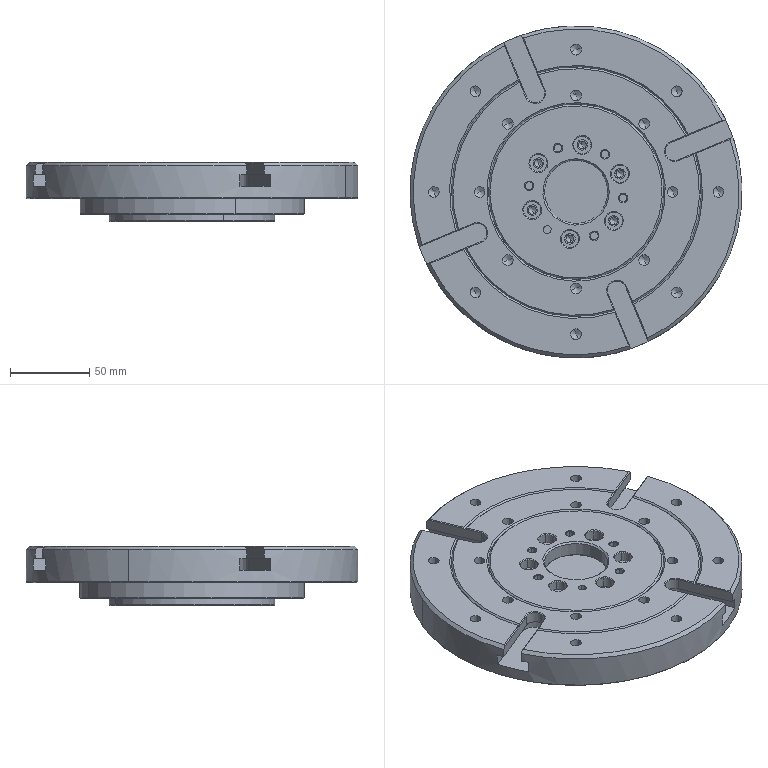NC program | Mastercam | posted with a generic post
Lines 1 to 959 of 19401:
%
:0001()
(MATERIAL - ALUMINUM MM - 2024)
(T1|25 BNOS |H1|D1|WEAR COMP|TOOL DIA. - 25.|XY STOCK TO LEAVE - .15|Z STOCK TO LEAVE - .1)
(T3|10 CHM |H3)
(T4|8.5 DR |H4)
(T5|14 FEM |H5)
(T6|6.8 DR |H6)
(T7|M8 X 1.25 RH |H7)
N100 G21
N102 G0 G17 G40 G80 G90 G94 G98
N104 G0 G28 G91 Z0.
N106 G0 G28 X0. Y0.
(25 BNOS |TOOL - 1|DIA. OFF. - 1|LEN. - 1|TOOL DIA. - 25.)
N108 T1 M6
N110 G0 G54 G90 X1.154 Y47.25 C0. B0. S2300 M3
N112 G43 H1 Z62.5
N114 Z14.2
N116 G1 Z12.708 F2000.
N118 G41 D1 Y28.5 F3500.
N120 Y8.5
N122 G40 Y-10.25
N124 Z12.215 F2000.
N126 G42 D1 Y8.5 F3500.
N128 Y28.5
N130 G40 Y47.25
N132 Z11.723 F2000.
N134 G41 D1 Y28.5 F3500.
N136 Y8.5
N138 G40 Y-10.25
N140 Z11.231 F2000.
N142 G42 D1 Y8.5 F3500.
N144 Y28.5
N146 G40 Y47.25
N148 Z10.738 F2000.
N150 G41 D1 Y28.5 F3500.
N152 Y8.5
N154 G40 Y-10.25
N156 Z10.246 F2000.
N158 G42 D1 Y8.5 F3500.
N160 Y28.5
N162 G40 Y47.25
N164 Z9.754 F2000.
N166 G41 D1 Y28.5 F3500.
N168 Y8.5
N170 G40 Y-10.25
N172 Z9.262 F2000.
N174 G42 D1 Y8.5 F3500.
N176 Y28.5
N178 G40 Y47.25
N180 Z8.769 F2000.
N182 G41 D1 Y28.5 F3500.
N184 Y8.5
N186 G40 Y-10.25
N188 Z8.277 F2000.
N190 G42 D1 Y8.5 F3500.
N192 Y28.5
N194 G40 Y47.25
N196 Z7.785 F2000.
N198 G41 D1 Y28.5 F3500.
N200 Y8.5
N202 G40 Y-10.25
N204 Z7.292 F2000.
N206 G42 D1 Y8.5 F3500.
N208 Y28.5
N210 G40 Y47.25
N212 Z6.8 F2000.
N214 G41 D1 Y28.5 F3500.
N216 Y8.5
N218 G40 Y-10.25
N220 Z6.308 F2000.
N222 G42 D1 Y8.5 F3500.
N224 Y28.5
N226 G40 Y47.25
N228 Z5.815 F2000.
N230 G41 D1 Y28.5 F3500.
N232 Y8.5
N234 G40 Y-10.25
N236 Z5.323 F2000.
N238 G42 D1 Y8.5 F3500.
N240 Y28.5
N242 G40 Y47.25
N244 Z4.831 F2000.
N246 G41 D1 Y28.5 F3500.
N248 Y8.5
N250 G40 Y-10.25
N252 Z4.338 F2000.
N254 G42 D1 Y8.5 F3500.
N256 Y28.5
N258 G40 Y47.25
N260 Z3.846 F2000.
N262 G41 D1 Y28.5 F3500.
N264 Y8.5
N266 G40 Y-10.25
N268 Z3.354 F2000.
N270 G42 D1 Y8.5 F3500.
N272 Y28.5
N274 G40 Y47.25
N276 Z2.862 F2000.
N278 G41 D1 Y28.5 F3500.
N280 Y8.5
N282 G40 Y-10.25
N284 Z2.369 F2000.
N286 G42 D1 Y8.5 F3500.
N288 Y28.5
N290 G40 Y47.25
N292 Z1.877 F2000.
N294 G41 D1 Y28.5 F3500.
N296 Y8.5
N298 G40 Y-10.25
N300 Z1.385 F2000.
N302 G42 D1 Y8.5 F3500.
N304 Y28.5
N306 G40 Y47.25
N308 Z.892 F2000.
N310 G41 D1 Y28.5 F3500.
N312 Y8.5
N314 G40 Y-10.25
N316 Z.4 F2000.
N318 G42 D1 Y8.5 F3500.
N320 Y28.5
N322 G40 Y47.25
N324 Z-.092 F2000.
N326 G41 D1 Y28.5 F3500.
N328 Y8.5
N330 G40 Y-10.25
N332 Z-.585 F2000.
N334 G42 D1 Y8.5 F3500.
N336 Y28.5
N338 G40 Y47.25
N340 Z-1.077 F2000.
N342 G41 D1 Y28.5 F3500.
N344 Y8.5
N346 G40 Y-10.25
N348 Z-1.569 F2000.
N350 G42 D1 Y8.5 F3500.
N352 Y28.5
N354 G40 Y47.25
N356 Z-2.062 F2000.
N358 G41 D1 Y28.5 F3500.
N360 Y8.5
N362 G40 Y-10.25
N364 Z-2.554 F2000.
N366 G42 D1 Y8.5 F3500.
N368 Y28.5
N370 G40 Y47.25
N372 Z-3.046 F2000.
N374 G41 D1 Y28.5 F3500.
N376 Y8.5
N378 G40 Y-10.25
N380 Z-3.538 F2000.
N382 G42 D1 Y8.5 F3500.
N384 Y28.5
N386 G40 Y47.25
N388 Z-4.031 F2000.
N390 G41 D1 Y28.5 F3500.
N392 Y8.5
N394 G40 Y-10.25
N396 Z-4.523 F2000.
N398 G42 D1 Y8.5 F3500.
N400 Y28.5
N402 G40 Y47.25
N404 Z-5.015 F2000.
N406 G41 D1 Y28.5 F3500.
N408 Y8.5
N410 G40 Y-10.25
N412 Z-5.508 F2000.
N414 G42 D1 Y8.5 F3500.
N416 Y28.5
N418 G40 Y47.25
N420 Z-6. F2000.
N422 G41 D1 Y28.5 F3500.
N424 Y8.5
N426 G40 Y-10.25
N428 Z-6.492 F2000.
N430 G42 D1 Y8.5 F3500.
N432 Y28.5
N434 G40 Y47.25
N436 Z-6.985 F2000.
N438 G41 D1 Y28.5 F3500.
N440 Y8.5
N442 G40 Y-10.25
N444 Z-7.477 F2000.
N446 G42 D1 Y8.5 F3500.
N448 Y28.5
N450 G40 Y47.25
N452 Z-7.969 F2000.
N454 G41 D1 Y28.5 F3500.
N456 Y8.5
N458 G40 Y-10.25
N460 Z-8.462 F2000.
N462 G42 D1 Y8.5 F3500.
N464 Y28.5
N466 G40 Y47.25
N468 Z-8.954 F2000.
N470 G41 D1 Y28.5 F3500.
N472 Y8.5
N474 G40 Y-10.25
N476 Z-9.446 F2000.
N478 G42 D1 Y8.5 F3500.
N480 Y28.5
N482 G40 Y47.25
N484 Z-9.938 F2000.
N486 G41 D1 Y28.5 F3500.
N488 Y8.5
N490 G40 Y-10.25
N492 Z-10.431 F2000.
N494 G42 D1 Y8.5 F3500.
N496 Y28.5
N498 G40 Y47.25
N500 Z-10.923 F2000.
N502 G41 D1 Y28.5 F3500.
N504 Y8.5
N506 G40 Y-10.25
N508 Z-11.415 F2000.
N510 G42 D1 Y8.5 F3500.
N512 Y28.5
N514 G40 Y47.25
N516 Z-11.908 F2000.
N518 G41 D1 Y28.5 F3500.
N520 Y8.5
N522 G40 Y-10.25
N524 Z-12.4 F2000.
N526 G42 D1 Y8.5 F3500.
N528 Y28.5
N530 G40 Y47.25
N532 G0 Z62.5
N534 S3500 M3
N536 X21.899 Y-5.5
N538 Z16.907
N540 G1 Z11.907 F2000.
N542 Y8.5
N544 Y28.5
N546 Y42.5
N548 X21.847
N550 Z11.715
N552 Y28.5
N554 Y8.5
N556 Y-5.5
N558 X21.795
N560 Z11.522
N562 Y8.5
N564 Y28.5
N566 Y42.5
N568 X21.744
N570 Z11.33
N572 Y28.5
N574 Y8.5
N576 Y-5.5
N578 X21.692
N580 Z11.138
N582 Y8.5
N584 Y28.5
N586 Y42.5
N588 X21.641
N590 Z10.946
N592 Y28.5
N594 Y8.5
N596 Y-5.5
N598 X21.589
N600 Z10.753
N602 Y8.5
N604 Y28.5
N606 Y42.5
N608 X21.538
N610 Z10.561
N612 Y28.5
N614 Y8.5
N616 Y-5.5
N618 X21.486
N620 Z10.369
N622 Y8.5
N624 Y28.5
N626 Y42.5
N628 X21.435
N630 Z10.176
N632 Y28.5
N634 Y8.5
N636 Y-5.5
N638 X21.383
N640 Z9.984
N642 Y8.5
N644 Y28.5
N646 Y42.5
N648 X21.332
N650 Z9.792
N652 Y28.5
N654 Y8.5
N656 Y-5.5
N658 X21.28
N660 Z9.599
N662 Y8.5
N664 Y28.5
N666 Y42.5
N668 X21.229
N670 Z9.407
N672 Y28.5
N674 Y8.5
N676 Y-5.5
N678 X21.177
N680 Z9.215
N682 Y8.5
N684 Y28.5
N686 Y42.5
N688 X21.126
N690 Z9.022
N692 Y28.5
N694 Y8.5
N696 Y-5.5
N698 X21.074
N700 Z8.83
N702 Y8.5
N704 Y28.5
N706 Y42.5
N708 X21.023
N710 Z8.638
N712 Y28.5
N714 Y8.5
N716 Y-5.5
N718 X20.971
N720 Z8.446
N722 Y8.5
N724 Y28.5
N726 Y42.5
N728 X20.919
N730 Z8.253
N732 Y28.5
N734 Y8.5
N736 Y-5.5
N738 X20.868
N740 Z8.061
N742 Y8.5
N744 Y28.5
N746 Y42.5
N748 X20.816
N750 Z7.869
N752 Y28.5
N754 Y8.5
N756 Y-5.5
N758 X20.765
N760 Z7.676
N762 Y8.5
N764 Y28.5
N766 Y42.5
N768 X20.713
N770 Z7.484
N772 Y28.5
N774 Y8.5
N776 Y-5.5
N778 X20.662
N780 Z7.292
N782 Y8.5
N784 Y28.5
N786 Y42.5
N788 X20.61
N790 Z7.099
N792 Y28.5
N794 Y8.5
N796 Y-5.5
N798 X20.559
N800 Z6.907
N802 Y8.5
N804 Y28.5
N806 Y42.5
N808 X20.507
N810 Z6.715
N812 Y28.5
N814 Y8.5
N816 Y-5.5
N818 X20.456
N820 Z6.522
N822 Y8.5
N824 Y28.5
N826 Y42.5
N828 X20.404
N830 Z6.33
N832 Y28.5
N834 Y8.5
N836 Y-5.5
N838 X20.353
N840 Z6.138
N842 Y8.5
N844 Y28.5
N846 Y42.5
N848 X20.301
N850 Z5.946
N852 Y28.5
N854 Y8.5
N856 Y-5.5
N858 X20.25
N860 Z5.753
N862 Y8.5
N864 Y28.5
N866 Y42.5
N868 X20.198
N870 Z5.561
N872 Y28.5
N874 Y8.5
N876 Y-5.5
N878 X20.147
N880 Z5.369
N882 Y8.5
N884 Y28.5
N886 Y42.5
N888 X20.095
N890 Z5.176
N892 Y28.5
N894 Y8.5
N896 Y-5.5
N898 X20.043
N900 Z4.984
N902 Y8.5
N904 Y28.5
N906 Y42.5
N908 X19.992
N910 Z4.792
N912 Y28.5
N914 Y8.5
N916 Y-5.5
N918 X19.94
N920 Z4.599
N922 Y8.5
N924 Y28.5
N926 Y42.5
N928 X19.889
N930 Z4.407
N932 Y28.5
N934 Y8.5
N936 Y-5.5
N938 X19.837
N940 Z4.215
N942 Y8.5
N944 Y28.5
N946 Y42.5
N948 X19.786
N950 Z4.022
N952 Y28.5
N954 Y8.5
N956 Y-5.5
N958 X19.734
N960 Z3.83
N962 Y8.5
N964 Y28.5
N966 Y42.5
N968 X19.683
N970 Z3.638
N972 Y28.5
N974 Y8.5
N976 Y-5.5
N978 X19.631
N980 Z3.446
N982 Y8.5
N984 Y28.5
N986 Y42.5
N988 X19.58
N990 Z3.253
N992 Y28.5
N994 Y8.5
N996 Y-5.5
N998 X19.528
N1000 Z3.061
N1002 Y8.5
N1004 Y28.5
N1006 Y42.5
N1008 X19.477
N1010 Z2.869
N1012 Y28.5
N1014 Y8.5
N1016 Y-5.5
N1018 X19.425
N1020 Z2.676
N1022 Y8.5
N1024 Y28.5
N1026 Y42.5
N1028 X19.374
N1030 Z2.484
N1032 Y28.5
N1034 Y8.5
N1036 Y-5.5
N1038 X19.322
N1040 Z2.292
N1042 Y8.5
N1044 Y28.5
N1046 Y42.5
N1048 X19.271
N1050 Z2.099
N1052 Y28.5
N1054 Y8.5
N1056 Y-5.5
N1058 X19.219
N1060 Z1.907
N1062 Y8.5
N1064 Y28.5
N1066 Y42.5
N1068 X19.168
N1070 Z1.715
N1072 Y28.5
N1074 Y8.5
N1076 Y-5.5
N1078 X19.116
N1080 Z1.522
N1082 Y8.5
N1084 Y28.5
N1086 Y42.5
N1088 X19.064
N1090 Z1.33
N1092 Y28.5
N1094 Y8.5
N1096 Y-5.5
N1098 X19.013
N1100 Z1.138
N1102 Y8.5
N1104 Y28.5
N1106 Y42.5
N1108 X18.961
N1110 Z.946
N1112 Y28.5
N1114 Y8.5
N1116 Y-5.5
N1118 X18.91
N1120 Z.753
N1122 Y8.5
N1124 Y28.5
N1126 Y42.5
N1128 X18.858
N1130 Z.561
N1132 Y28.5
N1134 Y8.5
N1136 Y-5.5
N1138 X18.807
N1140 Z.369
N1142 Y8.5
N1144 Y28.5
N1146 Y42.5
N1148 X18.755
N1150 Z.176
N1152 Y28.5
N1154 Y8.5
N1156 Y-5.5
N1158 X18.704
N1160 Z-.016
N1162 Y8.5
N1164 Y28.5
N1166 Y42.5
N1168 X18.652
N1170 Z-.208
N1172 Y28.5
N1174 Y8.5
N1176 Y-5.5
N1178 X18.601
N1180 Z-.401
N1182 Y8.5
N1184 Y28.5
N1186 Y42.5
N1188 X18.549
N1190 Z-.593
N1192 Y28.5
N1194 Y8.5
N1196 Y-5.5
N1198 X18.498
N1200 Z-.785
N1202 Y8.5
N1204 Y28.5
N1206 Y42.5
N1208 X18.446
N1210 Z-.978
N1212 Y28.5
N1214 Y8.5
N1216 Y-5.5
N1218 X18.395
N1220 Z-1.17
N1222 Y8.5
N1224 Y28.5
N1226 Y42.5
N1228 X18.343
N1230 Z-1.362
N1232 Y28.5
N1234 Y8.5
N1236 Y-5.5
N1238 X18.292
N1240 Z-1.554
N1242 Y8.5
N1244 Y28.5
N1246 Y42.5
N1248 X18.24
N1250 Z-1.747
N1252 Y28.5
N1254 Y8.5
N1256 Y-5.5
N1258 X18.188
N1260 Z-1.939
N1262 Y8.5
N1264 Y28.5
N1266 Y42.5
N1268 X18.137
N1270 Z-2.131
N1272 Y28.5
N1274 Y8.5
N1276 Y-5.5
N1278 X18.085
N1280 Z-2.324
N1282 Y8.5
N1284 Y28.5
N1286 Y42.5
N1288 X18.034
N1290 Z-2.516
N1292 Y28.5
N1294 Y8.5
N1296 Y-5.5
N1298 X17.982
N1300 Z-2.708
N1302 Y8.5
N1304 Y28.5
N1306 Y42.5
N1308 X17.931
N1310 Z-2.901
N1312 Y28.5
N1314 Y8.5
N1316 Y-5.5
N1318 X17.879
N1320 Z-3.093
N1322 Y8.5
N1324 Y28.5
N1326 Y42.5
N1328 X17.828
N1330 Z-3.285
N1332 Y28.5
N1334 Y8.5
N1336 Y-5.5
N1338 X17.776
N1340 Z-3.478
N1342 Y8.5
N1344 Y28.5
N1346 Y42.5
N1348 X17.725
N1350 Z-3.67
N1352 Y28.5
N1354 Y8.5
N1356 Y-5.5
N1358 X17.673
N1360 Z-3.862
N1362 Y8.5
N1364 Y28.5
N1366 Y42.5
N1368 X17.622
N1370 Z-4.054
N1372 Y28.5
N1374 Y8.5
N1376 Y-5.5
N1378 X17.57
N1380 Z-4.247
N1382 Y8.5
N1384 Y28.5
N1386 Y42.5
N1388 X17.519
N1390 Z-4.439
N1392 Y28.5
N1394 Y8.5
N1396 Y-5.5
N1398 X17.467
N1400 Z-4.631
N1402 Y8.5
N1404 Y28.5
N1406 Y42.5
N1408 X17.416
N1410 Z-4.824
N1412 Y28.5
N1414 Y8.5
N1416 Y-5.5
N1418 X17.364
N1420 Z-5.016
N1422 Y8.5
N1424 Y28.5
N1426 Y42.5
N1428 X17.312
N1430 Z-5.208
N1432 Y28.5
N1434 Y8.5
N1436 Y-5.5
N1438 X17.261
N1440 Z-5.401
N1442 Y8.5
N1444 Y28.5
N1446 Y42.5
N1448 X17.209
N1450 Z-5.593
N1452 Y28.5
N1454 Y8.5
N1456 Y-5.5
N1458 X17.158
N1460 Z-5.785
N1462 Y8.5
N1464 Y28.5
N1466 Y42.5
N1468 X17.106
N1470 Z-5.978
N1472 Y28.5
N1474 Y8.5
N1476 Y-5.5
N1478 X17.055
N1480 Z-6.17
N1482 Y8.5
N1484 Y28.5
N1486 Y42.5
N1488 X17.003
N1490 Z-6.362
N1492 Y28.5
N1494 Y8.5
N1496 Y-5.5
N1498 X16.952
N1500 Z-6.554
N1502 Y8.5
N1504 Y28.5
N1506 Y42.5
N1508 X16.9
N1510 Z-6.747
N1512 Y28.5
N1514 Y8.5
N1516 Y-5.5
N1518 X16.849
N1520 Z-6.939
N1522 Y8.5
N1524 Y28.5
N1526 Y42.5
N1528 X16.797
N1530 Z-7.131
N1532 Y28.5
N1534 Y8.5
N1536 Y-5.5
N1538 X16.746
N1540 Z-7.324
N1542 Y8.5
N1544 Y28.5
N1546 Y42.5
N1548 X16.694
N1550 Z-7.516
N1552 Y28.5
N1554 Y8.5
N1556 Y-5.5
N1558 X16.643
N1560 Z-7.708
N1562 Y8.5
N1564 Y28.5
N1566 Y42.5
N1568 X16.591
N1570 Z-7.901
N1572 Y28.5
N1574 Y8.5
N1576 Y-5.5
N1578 X16.54
N1580 Z-8.093
N1582 Y8.5
N1584 Y28.5
N1586 Y42.5
N1588 X16.488
N1590 Z-8.285
N1592 Y28.5
N1594 Y8.5
N1596 Y-5.5
N1598 X16.436
N1600 Z-8.478
N1602 Y8.5
N1604 Y28.5
N1606 Y42.5
N1608 X16.385
N1610 Z-8.67
N1612 Y28.5
N1614 Y8.5
N1616 Y-5.5
N1618 X16.333
N1620 Z-8.862
N1622 Y8.5
N1624 Y28.5
N1626 Y42.5
N1628 X16.282
N1630 Z-9.054
N1632 Y28.5
N1634 Y8.5
N1636 Y-5.5
N1638 X16.23
N1640 Z-9.247
N1642 Y8.5
N1644 Y28.5
N1646 Y42.5
N1648 X16.179
N1650 Z-9.439
N1652 Y28.5
N1654 Y8.5
N1656 Y-5.5
N1658 X16.127
N1660 Z-9.631
N1662 Y8.5
N1664 Y28.5
N1666 Y42.5
N1668 X16.076
N1670 Z-9.824
N1672 Y28.5
N1674 Y8.5
N1676 Y-5.5
N1678 X16.024
N1680 Z-10.016
N1682 Y8.5
N1684 Y28.5
N1686 Y42.5
N1688 X15.973
N1690 Z-10.208
N1692 Y28.5
N1694 Y8.5
N1696 Y-5.5
N1698 X15.921
N1700 Z-10.401
N1702 Y8.5
N1704 Y28.5
N1706 Y42.5
N1708 X15.87
N1710 Z-10.593
N1712 Y28.5
N1714 Y8.5
N1716 Y-5.5
N1718 X15.818
N1720 Z-10.785
N1722 Y8.5
N1724 Y28.5
N1726 Y42.5
N1728 X15.767
N1730 Z-10.978
N1732 Y28.5
N1734 Y8.5
N1736 Y-5.5
N1738 X15.715
N1740 Z-11.17
N1742 Y8.5
N1744 Y28.5
N1746 Y42.5
N1748 X15.664
N1750 Z-11.362
N1752 Y28.5
N1754 Y8.5
N1756 Y-5.5
N1758 X15.612
N1760 Z-11.554
N1762 Y8.5
N1764 Y28.5
N1766 Y42.5
N1768 X15.56
N1770 Z-11.747
N1772 Y28.5
N1774 Y8.5
N1776 Y-5.5
N1778 X15.509
N1780 Z-11.939
N1782 Y8.5
N1784 Y28.5
N1786 Y42.5
N1788 X15.457
N1790 Z-12.131
N1792 Y28.5
N1794 Y8.5
N1796 Y-5.5
N1798 X15.406
N1800 Z-12.324
N1802 Y8.5
N1804 Y28.5
N1806 Y42.5
N1808 G0 Z-7.324
N1810 Z62.5
N1812 X1.173 Y-10.25
N1814 Z14.2
N1816 G1 Z-12.5
N1818 G41 D1 Y8.5 F600.
N1820 Y28.5
N1822 G40 Y47.25
N1824 X15.173
N1826 G42 D1 Y28.5
N1828 Y8.5
N1830 G40 Y-10.25
N1832 G0 Z62.5
N1834 M5
N1836 G0 G28 G91 Z0.
N1838 G28
N1840 M01
N1842 G0 G17 G40 G80 G90 G94 G98
N1844 G0 G28 G91 Z0.
(10 CHM |TOOL - 3|DIA. OFF. - 3|LEN. - 3|TOOL DIA. - 10.)
N1846 T3 M6
N1848 G0 G54 G90 X-58.15 Y18.5 C0. B0. S2000 M3
N1850 G43 H3 Z62.5
N1852 G81 G98 Z10.5 R13.5 F100.
N1854 X63.85
N1856 X22.175 Z-14.5 R-11.5
N1858 G80
N1860 M5
N1862 G0 G28 G91 Z0.
N1864 G28
N1866 M01
N1868 G0 G17 G40 G80 G90 G94 G98
N1870 G0 G28 G91 Z0.
(8.5 DR |TOOL - 4|DIA. OFF. - 4|LEN. - 4|TOOL DIA. - 8.5)
N1872 T4 M6
N1874 G0 G54 G90 X-58.15 Y18.5 C0. B0. S1000 M3
N1876 G43 H4 Z62.5
N1878 G83 G98 Z-59.5 R13.5 Q5. F120.
N1880 X63.85
N1882 G80
N1884 M5
N1886 G0 G28 G91 Z0.
N1888 G28
N1890 M01
N1892 G0 G17 G40 G80 G90 G94 G98
N1894 G0 G28 G91 Z0.
(14 FEM |TOOL - 5|DIA. OFF. - 5|LEN. - 5|TOOL DIA. - 14.)
N1896 T5 M6
N1898 G0 G54 G90 X-58.15 Y18.5 C0. B0. S700 M3
N1900 G43 H5 Z62.5
N1902 G81 G98 Z-10.5 R13.5 F60.
N1904 X63.85
N1906 G80
N1908 M5
N1910 G0 G28 G91 Z0.
N1912 G28
N1914 M01
N1916 G0 G17 G40 G80 G90 G94 G98
N1918 G0 G28 G91 Z0.
(6.8 DR |TOOL - 6|DIA. OFF. - 6|LEN. - 6|TOOL DIA. - 6.8)
N1920 T6 M6
N1922 G0 G54 G90 X22.175 Y18.5 C0. B0. S1200 M3
N1924 G43 H6 Z62.5
N1926 G83 G98 Z-37.5 R-11.5 Q5. F150.
N1928 G80
N1930 M5
N1932 G0 G28 G91 Z0.
N1934 G28
N1936 M01
N1938 G0 G17 G40 G80 G90 G94 G98
N1940 G0 G28 G91 Z0.
(10 CHM |TOOL - 3|DIA. OFF. - 3|LEN. - 3|TOOL DIA. - 10.)
N1942 T3 M6
N1944 G0 G54 G90 X22.175 Y18.5 C0. B0. S1000 M3
N1946 G43 H3 Z62.5
N1948 G81 G98 Z-16.5 R-13.5 F200.
N1950 G80
N1952 M5
N1954 G0 G28 G91 Z0.
N1956 G28
N1958 M01
N1960 G0 G17 G40 G80 G90 G94 G98
N1962 G0 G28 G91 Z0.
(M8 X 1.25 RH |TOOL - 7|DIA. OFF. - 7|LEN. - 7|TOOL DIA. - 8.)
N1964 T7 M6
N1966 G0 G54 G90 X22.175 Y18.5 C0. B0. S200 M3
N1968 G43 H7 Z62.5
N1970 G84 G98 Z-17.5 R-11.5 F250.
N1972 G80
N1974 M5
N1976 G0 G28 G91 Z0.
N1978 G28
N1980 M01
N1982 G0 G17 G40 G80 G90 G94 G98
N1984 G0 G28 G91 Z0.